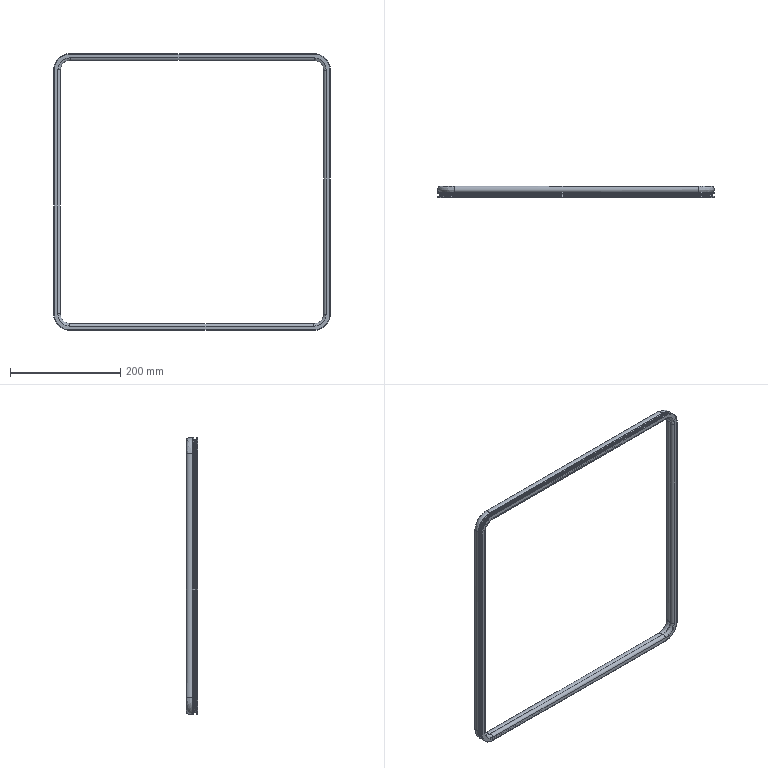Part | STEP file | 750038529 | 1 solid | 325 faces | box 501.538 x 20.12 x 501.538 mm | volume 180516 mm3 | spline 164 | cylinder 116 | plane 45 | commonest cylinder face diameters 0.6 x48 1 x32 2.05 x14 0.4 x12 5 x5 9.1 x5